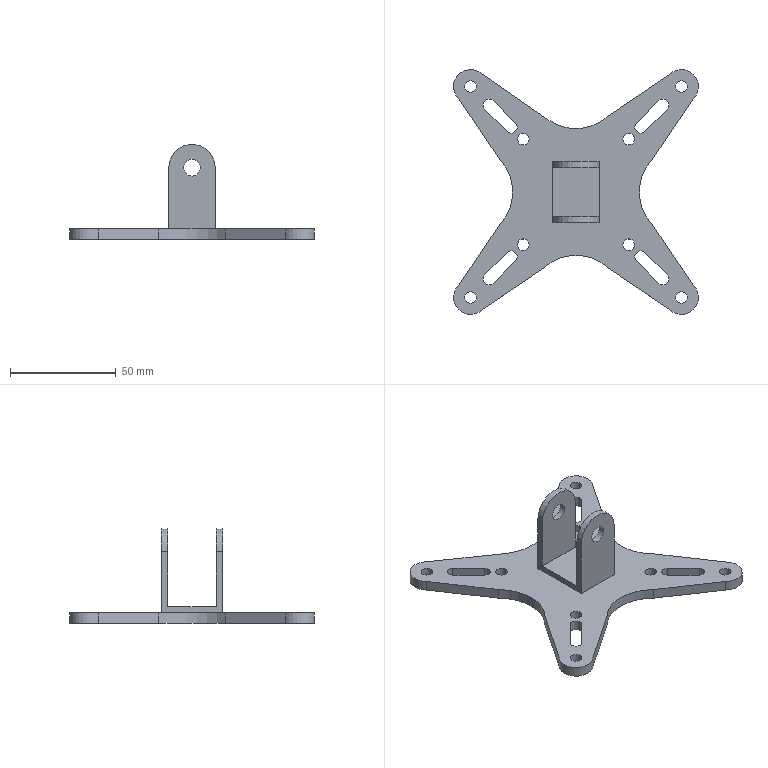Part | STEP file | 1 solid | 53 faces | box 116 x 116 x 45 mm | volume 39889 mm3 | cylinder 28 | plane 25 | commonest cylinder face diameters 5.5 x16 16 x4 45 x4 8 x2 22 x2